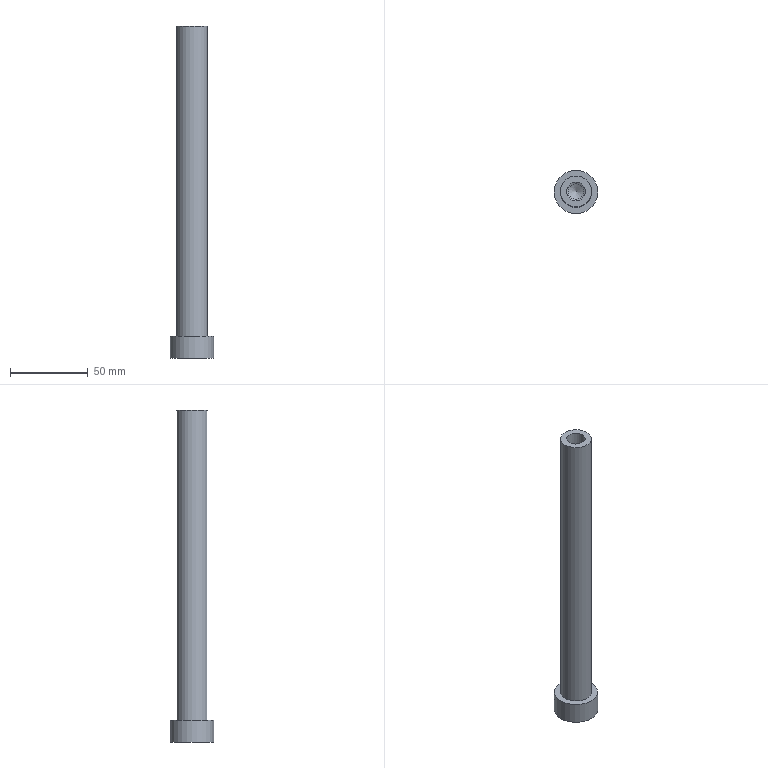Part | STEP file | 1_id538_xmt_txt | 1 solid | 16 faces | box 28 x 28 x 214 mm | volume 66281 mm3 | plane 10 | cylinder 4 | cone 2 | commonest cylinder face diameters 10.2 x1 12 x1 20 x1 28 x1
STEP:
#1=CARTESIAN_POINT('',(179.,235.,-113.));
#2=VERTEX_POINT('',#1);
#3=CARTESIAN_POINT('',(165.,235.,-113.));
#4=DIRECTION('',(0.,0.,-1.));
#5=DIRECTION('',(1.,0.,0.));
#6=AXIS2_PLACEMENT_3D('',#3,#4,#5);
#7=CIRCLE('',#6,14.);
#8=EDGE_CURVE('',#2,#2,#7,.T.);
#9=ORIENTED_EDGE('',*,*,#8,.F.);
#10=EDGE_LOOP('',(#9));
#11=FACE_BOUND('',#10,.T.);
#12=CARTESIAN_POINT('',(179.,235.,-99.));
#13=VERTEX_POINT('',#12);
#14=CARTESIAN_POINT('',(165.,235.,-99.));
#15=DIRECTION('',(0.,0.,1.));
#16=DIRECTION('',(1.,0.,0.));
#17=AXIS2_PLACEMENT_3D('',#14,#15,#16);
#18=CIRCLE('',#17,14.);
#19=EDGE_CURVE('',#13,#13,#18,.T.);
#20=ORIENTED_EDGE('',*,*,#19,.F.);
#21=EDGE_LOOP('',(#20));
#22=FACE_BOUND('',#21,.T.);
#23=CARTESIAN_POINT('',(165.,235.,-106.));
#24=DIRECTION('',(0.,0.,1.));
#25=DIRECTION('',(-1.,0.,0.));
#26=AXIS2_PLACEMENT_3D('',#23,#24,#25);
#27=CYLINDRICAL_SURFACE('',#26,14.);
#28=ADVANCED_FACE('',(#11,#22),#27,.T.);
#29=CARTESIAN_POINT('',(175.,235.,-99.));
#30=VERTEX_POINT('',#29);
#31=CARTESIAN_POINT('',(165.,235.,-99.));
#32=DIRECTION('',(0.,0.,-1.));
#33=DIRECTION('',(1.,0.,0.));
#34=AXIS2_PLACEMENT_3D('',#31,#32,#33);
#35=CIRCLE('',#34,10.);
#36=EDGE_CURVE('',#30,#30,#35,.T.);
#37=ORIENTED_EDGE('',*,*,#36,.F.);
#38=EDGE_LOOP('',(#37));
#39=FACE_BOUND('',#38,.T.);
#40=CARTESIAN_POINT('',(175.,235.,101.));
#41=VERTEX_POINT('',#40);
#42=CARTESIAN_POINT('',(165.,235.,101.));
#43=DIRECTION('',(0.,0.,1.));
#44=DIRECTION('',(1.,0.,0.));
#45=AXIS2_PLACEMENT_3D('',#42,#43,#44);
#46=CIRCLE('',#45,10.);
#47=EDGE_CURVE('',#41,#41,#46,.T.);
#48=ORIENTED_EDGE('',*,*,#47,.F.);
#49=EDGE_LOOP('',(#48));
#50=FACE_BOUND('',#49,.T.);
#51=CARTESIAN_POINT('',(165.,235.,1.));
#52=DIRECTION('',(0.,0.,1.));
#53=DIRECTION('',(-1.,0.,0.));
#54=AXIS2_PLACEMENT_3D('',#51,#52,#53);
#55=CYLINDRICAL_SURFACE('',#54,10.);
#56=ADVANCED_FACE('',(#39,#50),#55,.T.);
#57=CARTESIAN_POINT('',(159.,235.,71.));
#58=VERTEX_POINT('',#57);
#59=CARTESIAN_POINT('',(165.,235.,71.));
#60=DIRECTION('',(0.,0.,-1.));
#61=DIRECTION('',(-1.,0.,0.));
#62=AXIS2_PLACEMENT_3D('',#59,#60,#61);
#63=CIRCLE('',#62,6.);
#64=EDGE_CURVE('',#58,#58,#63,.T.);
#65=ORIENTED_EDGE('',*,*,#64,.T.);
#66=EDGE_LOOP('',(#65));
#67=FACE_BOUND('',#66,.T.);
#68=CARTESIAN_POINT('',(159.,235.,101.));
#69=VERTEX_POINT('',#68);
#70=CARTESIAN_POINT('',(165.,235.,101.));
#71=DIRECTION('',(0.,0.,-1.));
#72=DIRECTION('',(-1.,0.,0.));
#73=AXIS2_PLACEMENT_3D('',#70,#71,#72);
#74=CIRCLE('',#73,6.);
#75=EDGE_CURVE('',#69,#69,#74,.T.);
#76=ORIENTED_EDGE('',*,*,#75,.F.);
#77=EDGE_LOOP('',(#76));
#78=FACE_BOUND('',#77,.T.);
#79=CARTESIAN_POINT('',(165.,235.,86.));
#80=DIRECTION('',(0.,0.,-1.));
#81=DIRECTION('',(1.,0.,0.));
#82=AXIS2_PLACEMENT_3D('',#79,#80,#81);
#83=CYLINDRICAL_SURFACE('',#82,6.);
#84=ADVANCED_FACE('',(#67,#78),#83,.F.);
#85=CARTESIAN_POINT('',(159.9,235.,70.5));
#86=VERTEX_POINT('',#85);
#87=CARTESIAN_POINT('',(165.,235.,70.5));
#88=DIRECTION('',(0.,0.,-1.));
#89=DIRECTION('',(-1.,0.,0.));
#90=AXIS2_PLACEMENT_3D('',#87,#88,#89);
#91=CIRCLE('',#90,5.1);
#92=EDGE_CURVE('',#86,#86,#91,.T.);
#93=ORIENTED_EDGE('',*,*,#92,.T.);
#94=EDGE_LOOP('',(#93));
#95=FACE_BOUND('',#94,.T.);
#96=ORIENTED_EDGE('',*,*,#64,.F.);
#97=EDGE_LOOP('',(#96));
#98=FACE_BOUND('',#97,.T.);
#99=CARTESIAN_POINT('',(165.,235.,70.75));
#100=DIRECTION('',(0.,0.,1.));
#101=DIRECTION('',(1.,0.,0.));
#102=AXIS2_PLACEMENT_3D('',#99,#100,#101);
#103=CONICAL_SURFACE('',#102,5.55,60.945);
#104=ADVANCED_FACE('',(#95,#98),#103,.F.);
#105=CARTESIAN_POINT('',(159.9,235.,69.));
#106=VERTEX_POINT('',#105);
#107=CARTESIAN_POINT('',(165.,235.,69.));
#108=DIRECTION('',(0.,0.,-1.));
#109=DIRECTION('',(-1.,0.,0.));
#110=AXIS2_PLACEMENT_3D('',#107,#108,#109);
#111=CIRCLE('',#110,5.1);
#112=EDGE_CURVE('',#106,#106,#111,.T.);
#113=ORIENTED_EDGE('',*,*,#112,.T.);
#114=EDGE_LOOP('',(#113));
#115=FACE_BOUND('',#114,.T.);
#116=ORIENTED_EDGE('',*,*,#92,.F.);
#117=EDGE_LOOP('',(#116));
#118=FACE_BOUND('',#117,.T.);
#119=CARTESIAN_POINT('',(165.,235.,69.75));
#120=DIRECTION('',(0.,0.,-1.));
#121=DIRECTION('',(1.,0.,0.));
#122=AXIS2_PLACEMENT_3D('',#119,#120,#121);
#123=CYLINDRICAL_SURFACE('',#122,5.1);
#124=ADVANCED_FACE('',(#115,#118),#123,.F.);
#125=ORIENTED_EDGE('',*,*,#112,.F.);
#126=EDGE_LOOP('',(#125));
#127=FACE_BOUND('',#126,.T.);
#128=CARTESIAN_POINT('',(165.,235.,66.056));
#129=VERTEX_POINT('',#128);
#130=VERTEX_LOOP('',#129);
#131=FACE_BOUND('',#130,.T.);
#132=CARTESIAN_POINT('',(165.,235.,67.528));
#133=DIRECTION('',(0.,0.,1.));
#134=DIRECTION('',(1.,0.,0.));
#135=AXIS2_PLACEMENT_3D('',#132,#133,#134);
#136=CONICAL_SURFACE('',#135,2.55,60.);
#137=ADVANCED_FACE('',(#127,#131),#136,.F.);
#138=CARTESIAN_POINT('',(160.959,242.,-104.));
#139=VERTEX_POINT('',#138);
#140=CARTESIAN_POINT('',(169.041,242.,-104.));
#141=VERTEX_POINT('',#140);
#142=CARTESIAN_POINT('',(160.959,242.,-104.));
#143=DIRECTION('',(1.,0.,0.));
#144=VECTOR('',#143,1.);
#145=LINE('',#142,#144);
#146=EDGE_CURVE('',#139,#141,#145,.T.);
#147=ORIENTED_EDGE('',*,*,#146,.F.);
#148=CARTESIAN_POINT('',(160.959,242.,-113.));
#149=VERTEX_POINT('',#148);
#150=CARTESIAN_POINT('',(160.959,242.,-113.));
#151=DIRECTION('',(0.,0.,1.));
#152=VECTOR('',#151,1.);
#153=LINE('',#150,#152);
#154=EDGE_CURVE('',#149,#139,#153,.T.);
#155=ORIENTED_EDGE('',*,*,#154,.F.);
#156=CARTESIAN_POINT('',(169.041,242.,-113.));
#157=VERTEX_POINT('',#156);
#158=CARTESIAN_POINT('',(165.,242.,-113.));
#159=DIRECTION('',(-1.,0.,0.));
#160=VECTOR('',#159,1.);
#161=LINE('',#158,#160);
#162=EDGE_CURVE('',#157,#149,#161,.T.);
#163=ORIENTED_EDGE('',*,*,#162,.F.);
#164=CARTESIAN_POINT('',(169.041,242.,-113.));
#165=DIRECTION('',(0.,0.,1.));
#166=VECTOR('',#165,1.);
#167=LINE('',#164,#166);
#168=EDGE_CURVE('',#157,#141,#167,.T.);
#169=ORIENTED_EDGE('',*,*,#168,.T.);
#170=EDGE_LOOP('',(#147,#155,#163,#169));
#171=FACE_OUTER_BOUND('',#170,.T.);
#172=CARTESIAN_POINT('',(165.,242.,-113.));
#173=DIRECTION('',(0.,1.,0.));
#174=DIRECTION('',(1.,0.,0.));
#175=AXIS2_PLACEMENT_3D('',#172,#173,#174);
#176=PLANE('',#175);
#177=ADVANCED_FACE('',(#171),#176,.F.);
#178=CARTESIAN_POINT('',(173.083,235.,-104.));
#179=VERTEX_POINT('',#178);
#180=CARTESIAN_POINT('',(169.041,242.,-104.));
#181=DIRECTION('',(0.5,-0.866,0.));
#182=VECTOR('',#181,1.);
#183=LINE('',#180,#182);
#184=EDGE_CURVE('',#141,#179,#183,.T.);
#185=ORIENTED_EDGE('',*,*,#184,.F.);
#186=ORIENTED_EDGE('',*,*,#168,.F.);
#187=CARTESIAN_POINT('',(173.083,235.,-113.));
#188=VERTEX_POINT('',#187);
#189=CARTESIAN_POINT('',(171.062,238.5,-113.));
#190=DIRECTION('',(-0.5,0.866,0.));
#191=VECTOR('',#190,1.);
#192=LINE('',#189,#191);
#193=EDGE_CURVE('',#188,#157,#192,.T.);
#194=ORIENTED_EDGE('',*,*,#193,.F.);
#195=CARTESIAN_POINT('',(173.083,235.,-113.));
#196=DIRECTION('',(0.,0.,1.));
#197=VECTOR('',#196,1.);
#198=LINE('',#195,#197);
#199=EDGE_CURVE('',#188,#179,#198,.T.);
#200=ORIENTED_EDGE('',*,*,#199,.T.);
#201=EDGE_LOOP('',(#185,#186,#194,#200));
#202=FACE_OUTER_BOUND('',#201,.T.);
#203=CARTESIAN_POINT('',(171.062,238.5,-113.));
#204=DIRECTION('',(0.866,0.5,0.));
#205=DIRECTION('',(0.5,-0.866,0.));
#206=AXIS2_PLACEMENT_3D('',#203,#204,#205);
#207=PLANE('',#206);
#208=ADVANCED_FACE('',(#202),#207,.F.);
#209=CARTESIAN_POINT('',(169.041,228.,-104.));
#210=VERTEX_POINT('',#209);
#211=CARTESIAN_POINT('',(173.083,235.,-104.));
#212=DIRECTION('',(-0.5,-0.866,0.));
#213=VECTOR('',#212,1.);
#214=LINE('',#211,#213);
#215=EDGE_CURVE('',#179,#210,#214,.T.);
#216=ORIENTED_EDGE('',*,*,#215,.F.);
#217=ORIENTED_EDGE('',*,*,#199,.F.);
#218=CARTESIAN_POINT('',(169.041,228.,-113.));
#219=VERTEX_POINT('',#218);
#220=CARTESIAN_POINT('',(171.062,231.5,-113.));
#221=DIRECTION('',(0.5,0.866,0.));
#222=VECTOR('',#221,1.);
#223=LINE('',#220,#222);
#224=EDGE_CURVE('',#219,#188,#223,.T.);
#225=ORIENTED_EDGE('',*,*,#224,.F.);
#226=CARTESIAN_POINT('',(169.041,228.,-113.));
#227=DIRECTION('',(0.,0.,1.));
#228=VECTOR('',#227,1.);
#229=LINE('',#226,#228);
#230=EDGE_CURVE('',#219,#210,#229,.T.);
#231=ORIENTED_EDGE('',*,*,#230,.T.);
#232=EDGE_LOOP('',(#216,#217,#225,#231));
#233=FACE_OUTER_BOUND('',#232,.T.);
#234=CARTESIAN_POINT('',(171.062,231.5,-113.));
#235=DIRECTION('',(0.866,-0.5,0.));
#236=DIRECTION('',(-0.5,-0.866,0.));
#237=AXIS2_PLACEMENT_3D('',#234,#235,#236);
#238=PLANE('',#237);
#239=ADVANCED_FACE('',(#233),#238,.F.);
#240=CARTESIAN_POINT('',(160.959,228.,-104.));
#241=VERTEX_POINT('',#240);
#242=CARTESIAN_POINT('',(169.041,228.,-104.));
#243=DIRECTION('',(-1.,0.,0.));
#244=VECTOR('',#243,1.);
#245=LINE('',#242,#244);
#246=EDGE_CURVE('',#210,#241,#245,.T.);
#247=ORIENTED_EDGE('',*,*,#246,.F.);
#248=ORIENTED_EDGE('',*,*,#230,.F.);
#249=CARTESIAN_POINT('',(160.959,228.,-113.));
#250=VERTEX_POINT('',#249);
#251=CARTESIAN_POINT('',(165.,228.,-113.));
#252=DIRECTION('',(1.,0.,0.));
#253=VECTOR('',#252,1.);
#254=LINE('',#251,#253);
#255=EDGE_CURVE('',#250,#219,#254,.T.);
#256=ORIENTED_EDGE('',*,*,#255,.F.);
#257=CARTESIAN_POINT('',(160.959,228.,-113.));
#258=DIRECTION('',(0.,0.,1.));
#259=VECTOR('',#258,1.);
#260=LINE('',#257,#259);
#261=EDGE_CURVE('',#250,#241,#260,.T.);
#262=ORIENTED_EDGE('',*,*,#261,.T.);
#263=EDGE_LOOP('',(#247,#248,#256,#262));
#264=FACE_OUTER_BOUND('',#263,.T.);
#265=CARTESIAN_POINT('',(165.,228.,-113.));
#266=DIRECTION('',(0.,-1.,0.));
#267=DIRECTION('',(-1.,0.,0.));
#268=AXIS2_PLACEMENT_3D('',#265,#266,#267);
#269=PLANE('',#268);
#270=ADVANCED_FACE('',(#264),#269,.F.);
#271=CARTESIAN_POINT('',(156.917,235.,-104.));
#272=VERTEX_POINT('',#271);
#273=CARTESIAN_POINT('',(160.959,228.,-104.));
#274=DIRECTION('',(-0.5,0.866,0.));
#275=VECTOR('',#274,1.);
#276=LINE('',#273,#275);
#277=EDGE_CURVE('',#241,#272,#276,.T.);
#278=ORIENTED_EDGE('',*,*,#277,.F.);
#279=ORIENTED_EDGE('',*,*,#261,.F.);
#280=CARTESIAN_POINT('',(156.917,235.,-113.));
#281=VERTEX_POINT('',#280);
#282=CARTESIAN_POINT('',(158.938,231.5,-113.));
#283=DIRECTION('',(0.5,-0.866,0.));
#284=VECTOR('',#283,1.);
#285=LINE('',#282,#284);
#286=EDGE_CURVE('',#281,#250,#285,.T.);
#287=ORIENTED_EDGE('',*,*,#286,.F.);
#288=CARTESIAN_POINT('',(156.917,235.,-113.));
#289=DIRECTION('',(0.,0.,1.));
#290=VECTOR('',#289,1.);
#291=LINE('',#288,#290);
#292=EDGE_CURVE('',#281,#272,#291,.T.);
#293=ORIENTED_EDGE('',*,*,#292,.T.);
#294=EDGE_LOOP('',(#278,#279,#287,#293));
#295=FACE_OUTER_BOUND('',#294,.T.);
#296=CARTESIAN_POINT('',(158.938,231.5,-113.));
#297=DIRECTION('',(-0.866,-0.5,0.));
#298=DIRECTION('',(-0.5,0.866,0.));
#299=AXIS2_PLACEMENT_3D('',#296,#297,#298);
#300=PLANE('',#299);
#301=ADVANCED_FACE('',(#295),#300,.F.);
#302=CARTESIAN_POINT('',(156.917,235.,-104.));
#303=DIRECTION('',(0.5,0.866,0.));
#304=VECTOR('',#303,1.);
#305=LINE('',#302,#304);
#306=EDGE_CURVE('',#272,#139,#305,.T.);
#307=ORIENTED_EDGE('',*,*,#306,.F.);
#308=ORIENTED_EDGE('',*,*,#292,.F.);
#309=CARTESIAN_POINT('',(158.938,238.5,-113.));
#310=DIRECTION('',(-0.5,-0.866,0.));
#311=VECTOR('',#310,1.);
#312=LINE('',#309,#311);
#313=EDGE_CURVE('',#149,#281,#312,.T.);
#314=ORIENTED_EDGE('',*,*,#313,.F.);
#315=ORIENTED_EDGE('',*,*,#154,.T.);
#316=EDGE_LOOP('',(#307,#308,#314,#315));
#317=FACE_OUTER_BOUND('',#316,.T.);
#318=CARTESIAN_POINT('',(158.938,238.5,-113.));
#319=DIRECTION('',(-0.866,0.5,0.));
#320=DIRECTION('',(0.5,0.866,0.));
#321=AXIS2_PLACEMENT_3D('',#318,#319,#320);
#322=PLANE('',#321);
#323=ADVANCED_FACE('',(#317),#322,.F.);
#324=ORIENTED_EDGE('',*,*,#146,.T.);
#325=ORIENTED_EDGE('',*,*,#184,.T.);
#326=ORIENTED_EDGE('',*,*,#215,.T.);
#327=ORIENTED_EDGE('',*,*,#246,.T.);
#328=ORIENTED_EDGE('',*,*,#277,.T.);
#329=ORIENTED_EDGE('',*,*,#306,.T.);
#330=EDGE_LOOP('',(#324,#325,#326,#327,#328,#329));
#331=FACE_OUTER_BOUND('',#330,.T.);
#332=CARTESIAN_POINT('',(165.,235.,-104.));
#333=DIRECTION('',(0.,0.,1.));
#334=DIRECTION('',(-1.,0.,0.));
#335=AXIS2_PLACEMENT_3D('',#332,#333,#334);
#336=PLANE('',#335);
#337=ADVANCED_FACE('',(#331),#336,.F.);
#338=ORIENTED_EDGE('',*,*,#75,.T.);
#339=EDGE_LOOP('',(#338));
#340=FACE_BOUND('',#339,.T.);
#341=ORIENTED_EDGE('',*,*,#47,.T.);
#342=EDGE_LOOP('',(#341));
#343=FACE_BOUND('',#342,.T.);
#344=CARTESIAN_POINT('',(165.,235.,101.));
#345=DIRECTION('',(0.,0.,1.));
#346=DIRECTION('',(-1.,0.,0.));
#347=AXIS2_PLACEMENT_3D('',#344,#345,#346);
#348=PLANE('',#347);
#349=ADVANCED_FACE('',(#340,#343),#348,.T.);
#350=ORIENTED_EDGE('',*,*,#162,.T.);
#351=ORIENTED_EDGE('',*,*,#313,.T.);
#352=ORIENTED_EDGE('',*,*,#286,.T.);
#353=ORIENTED_EDGE('',*,*,#255,.T.);
#354=ORIENTED_EDGE('',*,*,#224,.T.);
#355=ORIENTED_EDGE('',*,*,#193,.T.);
#356=EDGE_LOOP('',(#350,#351,#352,#353,#354,#355));
#357=FACE_BOUND('',#356,.T.);
#358=ORIENTED_EDGE('',*,*,#8,.T.);
#359=EDGE_LOOP('',(#358));
#360=FACE_BOUND('',#359,.T.);
#361=CARTESIAN_POINT('',(165.,235.,-113.));
#362=DIRECTION('',(0.,0.,-1.));
#363=DIRECTION('',(1.,0.,0.));
#364=AXIS2_PLACEMENT_3D('',#361,#362,#363);
#365=PLANE('',#364);
#366=ADVANCED_FACE('',(#357,#360),#365,.T.);
#367=ORIENTED_EDGE('',*,*,#36,.T.);
#368=EDGE_LOOP('',(#367));
#369=FACE_BOUND('',#368,.T.);
#370=ORIENTED_EDGE('',*,*,#19,.T.);
#371=EDGE_LOOP('',(#370));
#372=FACE_BOUND('',#371,.T.);
#373=CARTESIAN_POINT('',(165.,235.,-99.));
#374=DIRECTION('',(0.,0.,1.));
#375=DIRECTION('',(-1.,0.,0.));
#376=AXIS2_PLACEMENT_3D('',#373,#374,#375);
#377=PLANE('',#376);
#378=ADVANCED_FACE('',(#369,#372),#377,.T.);
#379=CLOSED_SHELL('',(#28,#56,#84,#104,#124,#137,#177,#208,#239,#270,#301,#323,#337,#349,#366,#378));
#380=MANIFOLD_SOLID_BREP('',#379);
#381=(LENGTH_UNIT()NAMED_UNIT(*)SI_UNIT(.MILLI.,.METRE.));
#382=UNCERTAINTY_MEASURE_WITH_UNIT(LENGTH_MEASURE(0.00002),#381,'','');
#383=(NAMED_UNIT(*)PLANE_ANGLE_UNIT()SI_UNIT($,.RADIAN.));
#384=PLANE_ANGLE_MEASURE_WITH_UNIT(PLANE_ANGLE_MEASURE(0.01745),#383);
#385=DIMENSIONAL_EXPONENTS(0.,0.,0.,0.,0.,0.,0.);
#386=(CONVERSION_BASED_UNIT('DEGREE',#384)NAMED_UNIT(#385)PLANE_ANGLE_UNIT());
#387=(NAMED_UNIT(*)SI_UNIT($,.STERADIAN.)SOLID_ANGLE_UNIT());
#388=(GEOMETRIC_REPRESENTATION_CONTEXT(3)GLOBAL_UNCERTAINTY_ASSIGNED_CONTEXT((#382))GLOBAL_UNIT_ASSIGNED_CONTEXT((#381,#386,#387))REPRESENTATION_CONTEXT('',''));
#389=ADVANCED_BREP_SHAPE_REPRESENTATION('',(#380),#388);